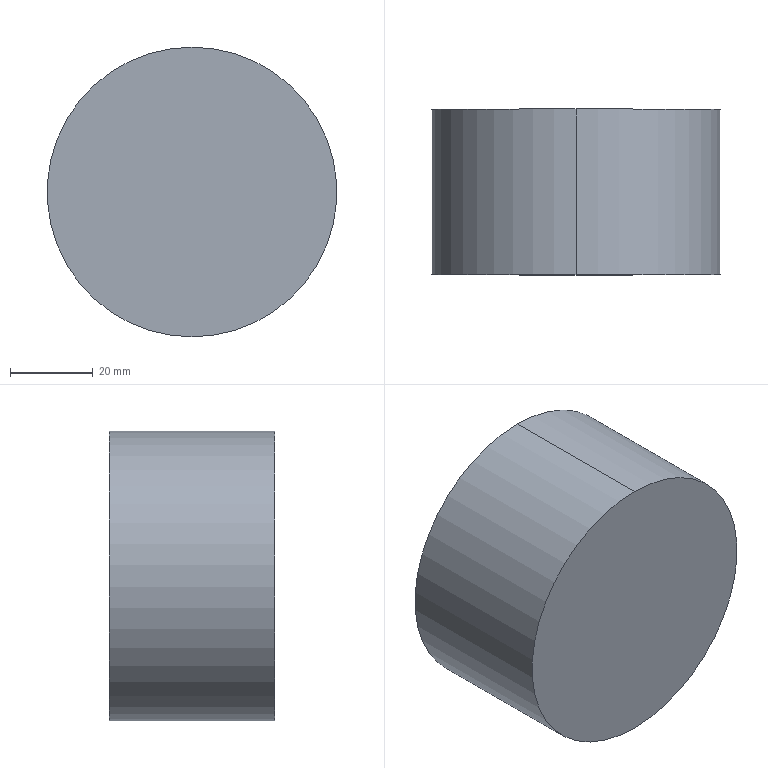Part | NX | 1 solid | 7 faces | box 70 x 40 x 70 mm | volume 34909 mm3 | cylinder 4 | plane 3 | commonest cylinder face diameters 64 x2 70 x2
STEP:
#1=CARTESIAN_POINT('',(0.,40.,32.));
#2=VERTEX_POINT('',#1);
#3=CARTESIAN_POINT('',(0.,40.,-32.));
#4=VERTEX_POINT('',#3);
#5=CARTESIAN_POINT('',(0.,40.,0.));
#6=DIRECTION('',(0.,-1.,0.));
#7=DIRECTION('',(0.,0.,-1.));
#8=AXIS2_PLACEMENT_3D('',#5,#6,#7);
#9=CIRCLE('',#8,32.);
#10=EDGE_CURVE('',#2,#4,#9,.T.);
#11=ORIENTED_EDGE('',*,*,#10,.F.);
#12=CARTESIAN_POINT('',(0.,3.,32.));
#13=VERTEX_POINT('',#12);
#14=CARTESIAN_POINT('',(0.,0.,32.));
#15=DIRECTION('',(0.,1.,0.));
#16=VECTOR('',#15,1.);
#17=LINE('',#14,#16);
#18=EDGE_CURVE('',#13,#2,#17,.T.);
#19=ORIENTED_EDGE('',*,*,#18,.F.);
#20=CARTESIAN_POINT('',(0.,3.,-32.));
#21=VERTEX_POINT('',#20);
#22=CARTESIAN_POINT('',(0.,3.,0.));
#23=DIRECTION('',(0.,-1.,0.));
#24=DIRECTION('',(0.,0.,-1.));
#25=AXIS2_PLACEMENT_3D('',#22,#23,#24);
#26=CIRCLE('',#25,32.);
#27=EDGE_CURVE('',#13,#21,#26,.T.);
#28=ORIENTED_EDGE('',*,*,#27,.T.);
#29=CARTESIAN_POINT('',(0.,0.,-32.));
#30=DIRECTION('',(0.,1.,0.));
#31=VECTOR('',#30,1.);
#32=LINE('',#29,#31);
#33=EDGE_CURVE('',#21,#4,#32,.T.);
#34=ORIENTED_EDGE('',*,*,#33,.T.);
#35=EDGE_LOOP('',(#11,#19,#28,#34));
#36=FACE_OUTER_BOUND('',#35,.T.);
#37=CARTESIAN_POINT('',(0.,0.,0.));
#38=DIRECTION('',(0.,-1.,0.));
#39=DIRECTION('',(0.,0.,-1.));
#40=AXIS2_PLACEMENT_3D('',#37,#38,#39);
#41=CYLINDRICAL_SURFACE('',#40,32.);
#42=ADVANCED_FACE('',(#36),#41,.F.);
#43=CARTESIAN_POINT('',(0.,40.,-35.));
#44=VERTEX_POINT('',#43);
#45=CARTESIAN_POINT('',(0.,40.,35.));
#46=VERTEX_POINT('',#45);
#47=CARTESIAN_POINT('',(0.,40.,0.));
#48=DIRECTION('',(0.,-1.,0.));
#49=DIRECTION('',(0.,0.,-1.));
#50=AXIS2_PLACEMENT_3D('',#47,#48,#49);
#51=CIRCLE('',#50,35.);
#52=EDGE_CURVE('',#44,#46,#51,.T.);
#53=ORIENTED_EDGE('',*,*,#52,.T.);
#54=CARTESIAN_POINT('',(0.,0.,35.));
#55=VERTEX_POINT('',#54);
#56=CARTESIAN_POINT('',(0.,0.,35.));
#57=DIRECTION('',(0.,1.,0.));
#58=VECTOR('',#57,1.);
#59=LINE('',#56,#58);
#60=EDGE_CURVE('',#55,#46,#59,.T.);
#61=ORIENTED_EDGE('',*,*,#60,.F.);
#62=CARTESIAN_POINT('',(0.,0.,-35.));
#63=VERTEX_POINT('',#62);
#64=CARTESIAN_POINT('',(0.,0.,0.));
#65=DIRECTION('',(0.,-1.,0.));
#66=DIRECTION('',(0.,0.,-1.));
#67=AXIS2_PLACEMENT_3D('',#64,#65,#66);
#68=CIRCLE('',#67,35.);
#69=EDGE_CURVE('',#63,#55,#68,.T.);
#70=ORIENTED_EDGE('',*,*,#69,.F.);
#71=CARTESIAN_POINT('',(0.,0.,-35.));
#72=DIRECTION('',(0.,1.,0.));
#73=VECTOR('',#72,1.);
#74=LINE('',#71,#73);
#75=EDGE_CURVE('',#63,#44,#74,.T.);
#76=ORIENTED_EDGE('',*,*,#75,.T.);
#77=EDGE_LOOP('',(#53,#61,#70,#76));
#78=FACE_OUTER_BOUND('',#77,.T.);
#79=CARTESIAN_POINT('',(0.,0.,0.));
#80=DIRECTION('',(0.,-1.,0.));
#81=DIRECTION('',(0.,0.,-1.));
#82=AXIS2_PLACEMENT_3D('',#79,#80,#81);
#83=CYLINDRICAL_SURFACE('',#82,35.);
#84=ADVANCED_FACE('',(#78),#83,.T.);
#85=ORIENTED_EDGE('',*,*,#69,.T.);
#86=CARTESIAN_POINT('',(0.,0.,0.));
#87=DIRECTION('',(0.,-1.,0.));
#88=DIRECTION('',(0.,0.,-1.));
#89=AXIS2_PLACEMENT_3D('',#86,#87,#88);
#90=CIRCLE('',#89,35.);
#91=EDGE_CURVE('',#55,#63,#90,.T.);
#92=ORIENTED_EDGE('',*,*,#91,.T.);
#93=EDGE_LOOP('',(#85,#92));
#94=FACE_OUTER_BOUND('',#93,.T.);
#95=CARTESIAN_POINT('',(0.,0.,0.));
#96=DIRECTION('',(0.,-1.,0.));
#97=DIRECTION('',(0.,0.,-1.));
#98=AXIS2_PLACEMENT_3D('',#95,#96,#97);
#99=PLANE('',#98);
#100=ADVANCED_FACE('',(#94),#99,.T.);
#101=ORIENTED_EDGE('',*,*,#60,.T.);
#102=CARTESIAN_POINT('',(0.,40.,0.));
#103=DIRECTION('',(0.,-1.,0.));
#104=DIRECTION('',(0.,0.,-1.));
#105=AXIS2_PLACEMENT_3D('',#102,#103,#104);
#106=CIRCLE('',#105,35.);
#107=EDGE_CURVE('',#46,#44,#106,.T.);
#108=ORIENTED_EDGE('',*,*,#107,.T.);
#109=ORIENTED_EDGE('',*,*,#75,.F.);
#110=ORIENTED_EDGE('',*,*,#91,.F.);
#111=EDGE_LOOP('',(#101,#108,#109,#110));
#112=FACE_OUTER_BOUND('',#111,.T.);
#113=CARTESIAN_POINT('',(0.,0.,0.));
#114=DIRECTION('',(0.,-1.,0.));
#115=DIRECTION('',(0.,0.,-1.));
#116=AXIS2_PLACEMENT_3D('',#113,#114,#115);
#117=CYLINDRICAL_SURFACE('',#116,35.);
#118=ADVANCED_FACE('',(#112),#117,.T.);
#119=CARTESIAN_POINT('',(0.,40.,0.));
#120=DIRECTION('',(0.,-1.,0.));
#121=DIRECTION('',(0.,0.,-1.));
#122=AXIS2_PLACEMENT_3D('',#119,#120,#121);
#123=CIRCLE('',#122,32.);
#124=EDGE_CURVE('',#4,#2,#123,.T.);
#125=ORIENTED_EDGE('',*,*,#124,.T.);
#126=ORIENTED_EDGE('',*,*,#10,.T.);
#127=EDGE_LOOP('',(#125,#126));
#128=FACE_BOUND('',#127,.T.);
#129=ORIENTED_EDGE('',*,*,#52,.F.);
#130=ORIENTED_EDGE('',*,*,#107,.F.);
#131=EDGE_LOOP('',(#129,#130));
#132=FACE_BOUND('',#131,.T.);
#133=CARTESIAN_POINT('',(32.,40.,0.));
#134=DIRECTION('',(0.,1.,0.));
#135=DIRECTION('',(0.,0.,1.));
#136=AXIS2_PLACEMENT_3D('',#133,#134,#135);
#137=PLANE('',#136);
#138=ADVANCED_FACE('',(#128,#132),#137,.T.);
#139=ORIENTED_EDGE('',*,*,#18,.T.);
#140=ORIENTED_EDGE('',*,*,#124,.F.);
#141=ORIENTED_EDGE('',*,*,#33,.F.);
#142=CARTESIAN_POINT('',(0.,3.,0.));
#143=DIRECTION('',(0.,-1.,0.));
#144=DIRECTION('',(0.,0.,-1.));
#145=AXIS2_PLACEMENT_3D('',#142,#143,#144);
#146=CIRCLE('',#145,32.);
#147=EDGE_CURVE('',#21,#13,#146,.T.);
#148=ORIENTED_EDGE('',*,*,#147,.T.);
#149=EDGE_LOOP('',(#139,#140,#141,#148));
#150=FACE_OUTER_BOUND('',#149,.T.);
#151=CARTESIAN_POINT('',(0.,0.,0.));
#152=DIRECTION('',(0.,-1.,0.));
#153=DIRECTION('',(0.,0.,-1.));
#154=AXIS2_PLACEMENT_3D('',#151,#152,#153);
#155=CYLINDRICAL_SURFACE('',#154,32.);
#156=ADVANCED_FACE('',(#150),#155,.F.);
#157=ORIENTED_EDGE('',*,*,#147,.F.);
#158=ORIENTED_EDGE('',*,*,#27,.F.);
#159=EDGE_LOOP('',(#157,#158));
#160=FACE_OUTER_BOUND('',#159,.T.);
#161=CARTESIAN_POINT('',(0.,3.,0.));
#162=DIRECTION('',(0.,1.,0.));
#163=DIRECTION('',(0.,0.,1.));
#164=AXIS2_PLACEMENT_3D('',#161,#162,#163);
#165=PLANE('',#164);
#166=ADVANCED_FACE('',(#160),#165,.T.);
#167=CLOSED_SHELL('',(#42,#84,#100,#118,#138,#156,#166));
#168=MANIFOLD_SOLID_BREP('',#167);
#169=(LENGTH_UNIT()NAMED_UNIT(*)SI_UNIT(.MILLI.,.METRE.));
#170=UNCERTAINTY_MEASURE_WITH_UNIT(LENGTH_MEASURE(0.00002),#169,'','');
#171=(NAMED_UNIT(*)PLANE_ANGLE_UNIT()SI_UNIT($,.RADIAN.));
#172=PLANE_ANGLE_MEASURE_WITH_UNIT(PLANE_ANGLE_MEASURE(0.01745),#171);
#173=DIMENSIONAL_EXPONENTS(0.,0.,0.,0.,0.,0.,0.);
#174=(CONVERSION_BASED_UNIT('DEGREE',#172)NAMED_UNIT(#173)PLANE_ANGLE_UNIT());
#175=(NAMED_UNIT(*)SI_UNIT($,.STERADIAN.)SOLID_ANGLE_UNIT());
#176=(GEOMETRIC_REPRESENTATION_CONTEXT(3)GLOBAL_UNCERTAINTY_ASSIGNED_CONTEXT((#170))GLOBAL_UNIT_ASSIGNED_CONTEXT((#169,#174,#175))REPRESENTATION_CONTEXT('',''));
#177=ADVANCED_BREP_SHAPE_REPRESENTATION('',(#168),#176);